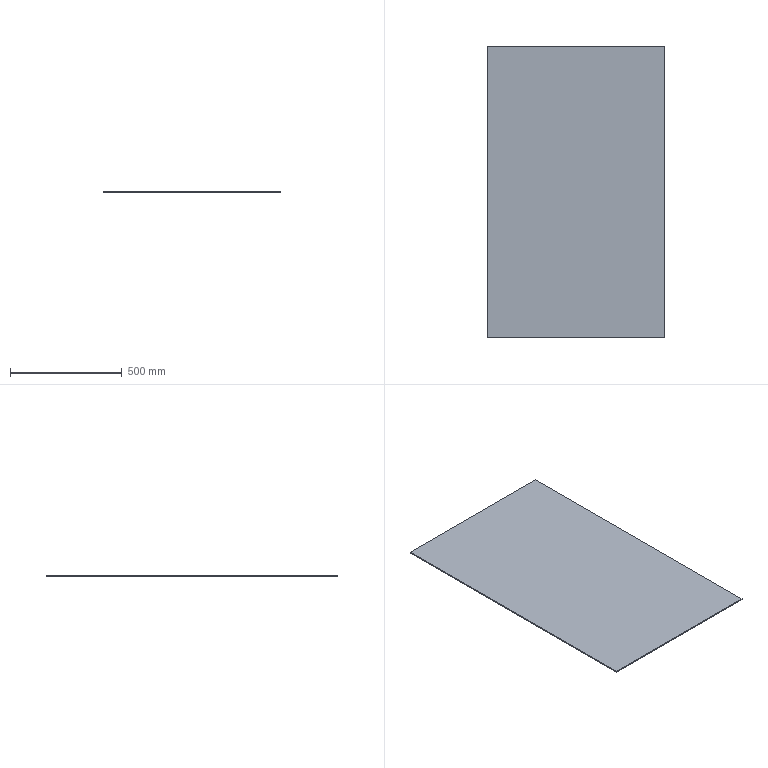Part | SolidWorks | features Extrusion 1, HoleWzd 1 | 1 solid | 6 faces | box 794 x 1306 x 5 mm | volume 5184820 mm3 | plane 6
STEP:
#1=CARTESIAN_POINT('',(397.,-653.,0.));
#2=VERTEX_POINT('',#1);
#3=CARTESIAN_POINT('',(397.,653.,0.));
#4=VERTEX_POINT('',#3);
#5=CARTESIAN_POINT('',(397.,653.,0.));
#6=DIRECTION('',(0.,1.,0.));
#7=VECTOR('',#6,1000.);
#8=LINE('',#5,#7);
#9=EDGE_CURVE('',#2,#4,#8,.T.);
#10=ORIENTED_EDGE('',*,*,#9,.T.);
#11=CARTESIAN_POINT('',(397.,653.,5.));
#12=VERTEX_POINT('',#11);
#13=CARTESIAN_POINT('',(397.,653.,5.));
#14=DIRECTION('',(0.,0.,-1.));
#15=VECTOR('',#14,1000.);
#16=LINE('',#13,#15);
#17=EDGE_CURVE('',#12,#4,#16,.T.);
#18=ORIENTED_EDGE('',*,*,#17,.F.);
#19=CARTESIAN_POINT('',(397.,-653.,5.));
#20=VERTEX_POINT('',#19);
#21=CARTESIAN_POINT('',(397.,653.,5.));
#22=DIRECTION('',(0.,1.,0.));
#23=VECTOR('',#22,1000.);
#24=LINE('',#21,#23);
#25=EDGE_CURVE('',#20,#12,#24,.T.);
#26=ORIENTED_EDGE('',*,*,#25,.F.);
#27=CARTESIAN_POINT('',(397.,-653.,5.));
#28=DIRECTION('',(0.,0.,-1.));
#29=VECTOR('',#28,1000.);
#30=LINE('',#27,#29);
#31=EDGE_CURVE('',#20,#2,#30,.T.);
#32=ORIENTED_EDGE('',*,*,#31,.T.);
#33=EDGE_LOOP('',(#10,#18,#26,#32));
#34=FACE_OUTER_BOUND('',#33,.T.);
#35=CARTESIAN_POINT('',(397.,653.,5.));
#36=DIRECTION('',(-1.,0.,0.));
#37=DIRECTION('',(0.,-1.,0.));
#38=AXIS2_PLACEMENT_3D('',#35,#36,#37);
#39=PLANE('',#38);
#40=ADVANCED_FACE('',(#34),#39,.F.);
#41=CARTESIAN_POINT('',(-397.,653.,0.));
#42=VERTEX_POINT('',#41);
#43=CARTESIAN_POINT('',(-397.,653.,0.));
#44=DIRECTION('',(-1.,0.,0.));
#45=VECTOR('',#44,1000.);
#46=LINE('',#43,#45);
#47=EDGE_CURVE('',#4,#42,#46,.T.);
#48=ORIENTED_EDGE('',*,*,#47,.T.);
#49=CARTESIAN_POINT('',(-397.,653.,5.));
#50=VERTEX_POINT('',#49);
#51=CARTESIAN_POINT('',(-397.,653.,5.));
#52=DIRECTION('',(0.,0.,-1.));
#53=VECTOR('',#52,1000.);
#54=LINE('',#51,#53);
#55=EDGE_CURVE('',#50,#42,#54,.T.);
#56=ORIENTED_EDGE('',*,*,#55,.F.);
#57=CARTESIAN_POINT('',(-397.,653.,5.));
#58=DIRECTION('',(-1.,0.,0.));
#59=VECTOR('',#58,1000.);
#60=LINE('',#57,#59);
#61=EDGE_CURVE('',#12,#50,#60,.T.);
#62=ORIENTED_EDGE('',*,*,#61,.F.);
#63=ORIENTED_EDGE('',*,*,#17,.T.);
#64=EDGE_LOOP('',(#48,#56,#62,#63));
#65=FACE_OUTER_BOUND('',#64,.T.);
#66=CARTESIAN_POINT('',(-397.,653.,5.));
#67=DIRECTION('',(0.,-1.,0.));
#68=DIRECTION('',(0.,0.,-1.));
#69=AXIS2_PLACEMENT_3D('',#66,#67,#68);
#70=PLANE('',#69);
#71=ADVANCED_FACE('',(#65),#70,.F.);
#72=CARTESIAN_POINT('',(-397.,-653.,0.));
#73=VERTEX_POINT('',#72);
#74=CARTESIAN_POINT('',(-397.,653.,0.));
#75=DIRECTION('',(0.,-1.,0.));
#76=VECTOR('',#75,1000.);
#77=LINE('',#74,#76);
#78=EDGE_CURVE('',#42,#73,#77,.T.);
#79=ORIENTED_EDGE('',*,*,#78,.T.);
#80=CARTESIAN_POINT('',(-397.,-653.,5.));
#81=VERTEX_POINT('',#80);
#82=CARTESIAN_POINT('',(-397.,-653.,5.));
#83=DIRECTION('',(0.,0.,-1.));
#84=VECTOR('',#83,1000.);
#85=LINE('',#82,#84);
#86=EDGE_CURVE('',#81,#73,#85,.T.);
#87=ORIENTED_EDGE('',*,*,#86,.F.);
#88=CARTESIAN_POINT('',(-397.,653.,5.));
#89=DIRECTION('',(0.,-1.,0.));
#90=VECTOR('',#89,1000.);
#91=LINE('',#88,#90);
#92=EDGE_CURVE('',#50,#81,#91,.T.);
#93=ORIENTED_EDGE('',*,*,#92,.F.);
#94=ORIENTED_EDGE('',*,*,#55,.T.);
#95=EDGE_LOOP('',(#79,#87,#93,#94));
#96=FACE_OUTER_BOUND('',#95,.T.);
#97=CARTESIAN_POINT('',(-397.,653.,5.));
#98=DIRECTION('',(1.,0.,0.));
#99=DIRECTION('',(0.,1.,0.));
#100=AXIS2_PLACEMENT_3D('',#97,#98,#99);
#101=PLANE('',#100);
#102=ADVANCED_FACE('',(#96),#101,.F.);
#103=CARTESIAN_POINT('',(-397.,-653.,0.));
#104=DIRECTION('',(1.,0.,0.));
#105=VECTOR('',#104,1000.);
#106=LINE('',#103,#105);
#107=EDGE_CURVE('',#73,#2,#106,.T.);
#108=ORIENTED_EDGE('',*,*,#107,.T.);
#109=ORIENTED_EDGE('',*,*,#31,.F.);
#110=CARTESIAN_POINT('',(-397.,-653.,5.));
#111=DIRECTION('',(1.,0.,0.));
#112=VECTOR('',#111,1000.);
#113=LINE('',#110,#112);
#114=EDGE_CURVE('',#81,#20,#113,.T.);
#115=ORIENTED_EDGE('',*,*,#114,.F.);
#116=ORIENTED_EDGE('',*,*,#86,.T.);
#117=EDGE_LOOP('',(#108,#109,#115,#116));
#118=FACE_OUTER_BOUND('',#117,.T.);
#119=CARTESIAN_POINT('',(-397.,-653.,5.));
#120=DIRECTION('',(0.,1.,0.));
#121=DIRECTION('',(0.,0.,1.));
#122=AXIS2_PLACEMENT_3D('',#119,#120,#121);
#123=PLANE('',#122);
#124=ADVANCED_FACE('',(#118),#123,.F.);
#125=ORIENTED_EDGE('',*,*,#25,.T.);
#126=ORIENTED_EDGE('',*,*,#61,.T.);
#127=ORIENTED_EDGE('',*,*,#92,.T.);
#128=ORIENTED_EDGE('',*,*,#114,.T.);
#129=EDGE_LOOP('',(#125,#126,#127,#128));
#130=FACE_OUTER_BOUND('',#129,.T.);
#131=CARTESIAN_POINT('',(0.,0.,5.));
#132=DIRECTION('',(0.,0.,1.));
#133=DIRECTION('',(1.,0.,0.));
#134=AXIS2_PLACEMENT_3D('',#131,#132,#133);
#135=PLANE('',#134);
#136=ADVANCED_FACE('',(#130),#135,.T.);
#137=ORIENTED_EDGE('',*,*,#9,.F.);
#138=ORIENTED_EDGE('',*,*,#107,.F.);
#139=ORIENTED_EDGE('',*,*,#78,.F.);
#140=ORIENTED_EDGE('',*,*,#47,.F.);
#141=EDGE_LOOP('',(#137,#138,#139,#140));
#142=FACE_OUTER_BOUND('',#141,.T.);
#143=CARTESIAN_POINT('',(0.,0.,0.));
#144=DIRECTION('',(0.,0.,1.));
#145=DIRECTION('',(1.,0.,0.));
#146=AXIS2_PLACEMENT_3D('',#143,#144,#145);
#147=PLANE('',#146);
#148=ADVANCED_FACE('',(#142),#147,.F.);
#149=CLOSED_SHELL('',(#40,#71,#102,#124,#136,#148));
#150=MANIFOLD_SOLID_BREP('',#149);
#151=CARTESIAN_POINT('',(0.,0.,0.));
#152=DIRECTION('',(0.,0.,1.));
#153=DIRECTION('',(1.,0.,0.));
#154=AXIS2_PLACEMENT_3D('',#151,#152,#153);
#155=(LENGTH_UNIT()NAMED_UNIT(*)SI_UNIT(.MILLI.,.METRE.));
#156=UNCERTAINTY_MEASURE_WITH_UNIT(LENGTH_MEASURE(0.00001),#155,'','');
#157=(NAMED_UNIT(*)PLANE_ANGLE_UNIT()SI_UNIT($,.RADIAN.));
#158=(NAMED_UNIT(*)SI_UNIT($,.STERADIAN.)SOLID_ANGLE_UNIT());
#159=(GEOMETRIC_REPRESENTATION_CONTEXT(3)GLOBAL_UNCERTAINTY_ASSIGNED_CONTEXT((#156))GLOBAL_UNIT_ASSIGNED_CONTEXT((#155,#157,#158))REPRESENTATION_CONTEXT('',''));
#160=ADVANCED_BREP_SHAPE_REPRESENTATION('',(#150,#154),#159);